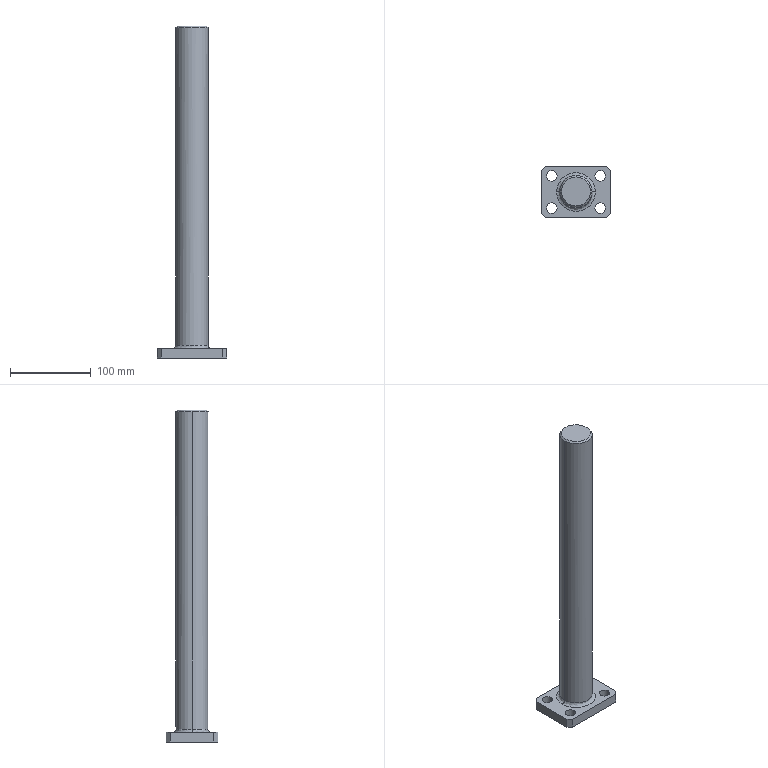Part | STEP file | 1 solid | 25 faces | box 86 x 64 x 412 mm | volume 562004 mm3 | plane 11 | cylinder 10 | cone 2 | spline 2 | commonest cylinder face diameters 13 x8 40 x2